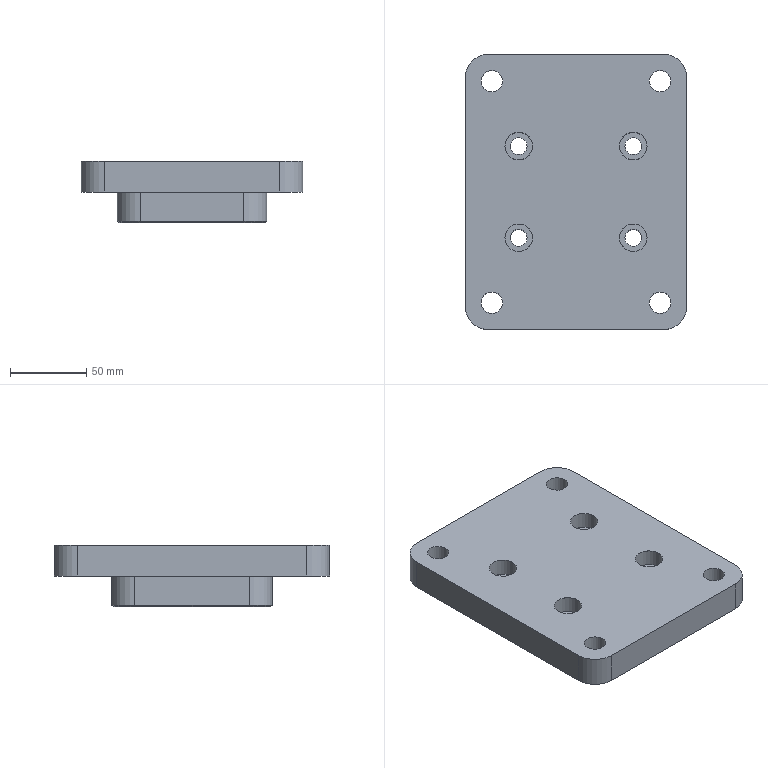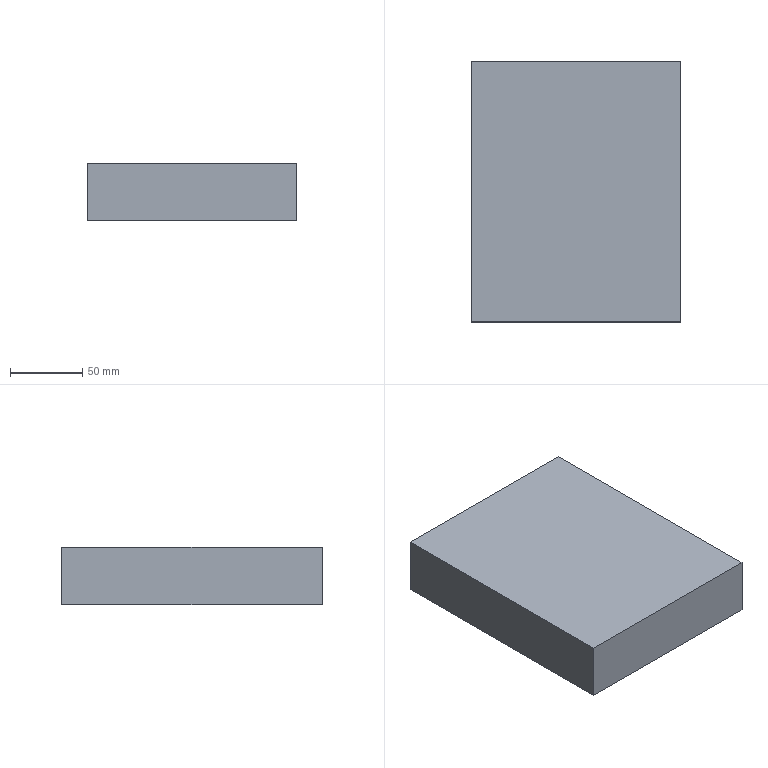CAM job | NX | 3-axis milling, drilling | part box 145 x 180 x 40 mm | stock box 145 x 180 x 40 mm
Tools:
number,name,description,diameter,corner_radius,flute_length,length,flutes
1,ZXZ,Milling Tool-5 Parameters,6.0,0.0,50.0,75.0,2
13,11.0ZT,Drilling Tool,11.0,0.0,35.0,50.0,2
10,D10,Milling Tool-5 Parameters,10.0,0.0,50.0,75.0,2
11,D10JING,Milling Tool-5 Parameters,10.0,0.0,50.0,75.0,2
7,D6A45,Milling Tool-5 Parameters,6.0,0.0,50.0,75.0,2
2,D50,Milling Tool-5 Parameters,50.0,0.0,50.0,75.0,2
Operations:
program,operation,operation_type,tool,method,geometry_group,spindle_rpm,surface_speed,feed_per_tooth,feed_cut,feed_plunge,cut_length_mm,path_length_mm,cut_time_min,machine_time_min
1,DRILLING,Operation,ZXZ,METHOD,A,5000.0,94.0,0.025,250.0,0.0,32.0,559.43,0.128,0.1807
1,DRILLING_COPY,Operation,11.0ZT,METHOD,A,2000.0,84.0,0.05,200.0,0.0,302.438,1100.305,1.512,1.592
1,ZLEVEL_PROFILE_1_COPY,ZLevelMilling,D10,METHOD,A,3200.0,100.0,0.3438,2200.0,100.0,16191.584,44295.105,7.36,10.17
1,HOLE_MILLING,CylinderMilling,D10,METHOD,A,3200.0,100.0,0.3438,2200.0,100.0,10954.96,12012.791,4.979,5.085
1,HOLE_MILLING_COPY,CylinderMilling,D10JING,METHOD,A,5000.0,157.0,0.12,1200.0,100.0,681.474,1695.322,0.5679,0.6693
1,ZLEVEL_PROFILE_1,ZLevelMilling,D10JING,METHOD,A,5000.0,157.0,0.125,1250.0,100.0,207.043,1103.043,0.1656,0.2552
1,PLANAR_MILL_COPY_COPY,PlanarMilling,D6A45,METHOD,A,7500.0,141.0,0.0833,1250.0,100.0,1039.531,1989.222,0.8316,0.9266
2,ZLEVEL_PROFILE_COPY_COPY,ZLevelMilling,D50,METHOD,B,1200.0,188.0,0.625,1500.0,1000.0,30832.299,30906.149,20.598,20.605
2,FLOOR_WALL,VolumeBased25DMillingOperation,D10JING,METHOD,B,5000.0,157.0,0.12,1200.0,500.0,3956.987,4456.1,3.212,3.262
2,PLANAR_MILL_COPY_COPY_COPY,PlanarMilling,D6A45,METHOD,B,7500.0,141.0,0.0833,1250.0,100.0,532.7,1063.302,0.4262,0.4792
2,PLANAR_MILL_COPY_COPY_COPY_COPY,PlanarMilling,D6A45,METHOD,B,7500.0,141.0,0.0833,1250.0,100.0,804.974,1675.503,0.644,0.731